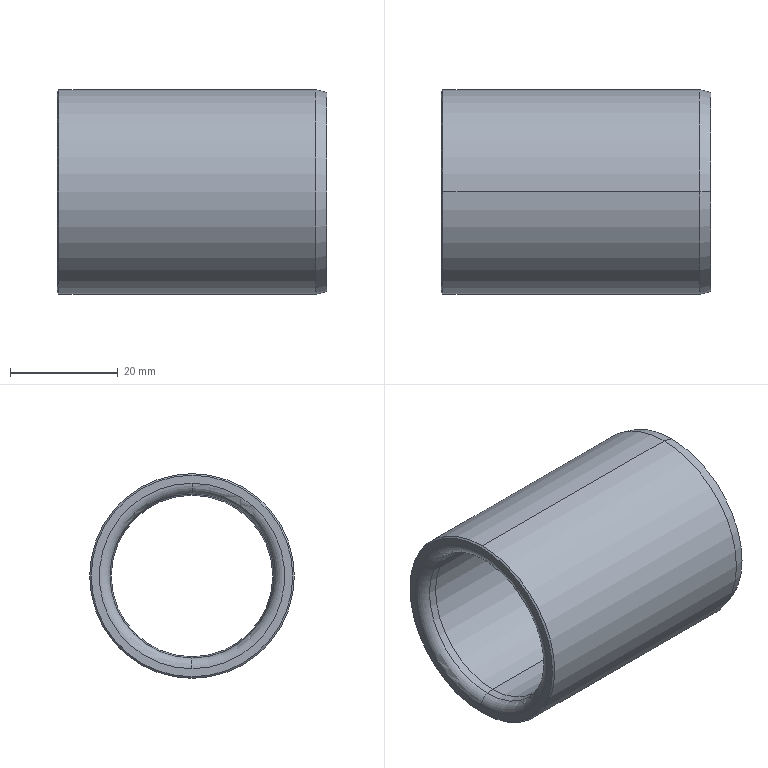Part | STEP file | MPBZ30_50_MPBZ30-50 | 1 solid | 18 faces | box 50 x 38 x 38 mm | volume 21031 mm3 | cone 8 | cylinder 4 | torus 4 | plane 2 | commonest cylinder face diameters 30 x2 38 x2
STEP:
#1=CARTESIAN_POINT('',(0.,0.,0.));
#2=DIRECTION('',(0.,0.,1.));
#3=DIRECTION('',(1.,0.,0.));
#4=AXIS2_PLACEMENT_3D('',#1,#2,#3);
#5=CARTESIAN_POINT('',(48.,0.,19.));
#6=VERTEX_POINT('',#5);
#7=CARTESIAN_POINT('',(48.,0.,-19.));
#8=VERTEX_POINT('',#7);
#9=CARTESIAN_POINT('',(48.,0.,0.));
#10=DIRECTION('',(-1.,0.,0.));
#11=DIRECTION('',(0.,0.,1.));
#12=AXIS2_PLACEMENT_3D('',#9,#10,#11);
#13=CIRCLE('',#12,19.);
#14=CARTESIAN_POINT('',(50.,0.,0.));
#15=DIRECTION('',(-1.,0.,0.));
#16=DIRECTION('',(0.,0.,1.));
#17=AXIS2_PLACEMENT_3D('',#14,#15,#16);
#18=CYLINDRICAL_SURFACE('',#17,19.);
#19=CARTESIAN_POINT('',(0.,2.));
#20=DIRECTION('',(1.,0.));
#21=VECTOR('',#20,1.);
#22=LINE('',#19,#21);
#23=(GEOMETRIC_REPRESENTATION_CONTEXT(2)PARAMETRIC_REPRESENTATION_CONTEXT()REPRESENTATION_CONTEXT('',''));
#24=DEFINITIONAL_REPRESENTATION('',(#22),#23);
#25=PCURVE('',#18,#24);
#26=CARTESIAN_POINT('',(50.,0.,0.));
#27=DIRECTION('',(-1.,0.,0.));
#28=DIRECTION('',(0.,0.,1.));
#29=AXIS2_PLACEMENT_3D('',#26,#27,#28);
#30=CONICAL_SURFACE('',#29,18.464,0.2618);
#31=CARTESIAN_POINT('',(0.,2.));
#32=DIRECTION('',(1.,0.));
#33=VECTOR('',#32,1.);
#34=LINE('',#31,#33);
#35=(GEOMETRIC_REPRESENTATION_CONTEXT(2)PARAMETRIC_REPRESENTATION_CONTEXT()REPRESENTATION_CONTEXT('',''));
#36=DEFINITIONAL_REPRESENTATION('',(#34),#35);
#37=PCURVE('',#30,#36);
#38=SURFACE_CURVE('',#13,(#25,#37),.PCURVE_S1.);
#39=EDGE_CURVE('',#6,#8,#38,.T.);
#40=ORIENTED_EDGE('',*,*,#39,.T.);
#41=CARTESIAN_POINT('',(0.3,0.,-19.));
#42=VERTEX_POINT('',#41);
#43=CARTESIAN_POINT('',(50.,0.,-19.));
#44=DIRECTION('',(-1.,0.,0.));
#45=VECTOR('',#44,1.);
#46=LINE('',#43,#45);
#47=CARTESIAN_POINT('',(3.142,0.));
#48=DIRECTION('',(0.,1.));
#49=VECTOR('',#48,1.);
#50=LINE('',#47,#49);
#51=(GEOMETRIC_REPRESENTATION_CONTEXT(2)PARAMETRIC_REPRESENTATION_CONTEXT()REPRESENTATION_CONTEXT('',''));
#52=DEFINITIONAL_REPRESENTATION('',(#50),#51);
#53=PCURVE('',#18,#52);
#54=CARTESIAN_POINT('',(50.,0.,0.));
#55=DIRECTION('',(-1.,0.,0.));
#56=DIRECTION('',(0.,0.,1.));
#57=AXIS2_PLACEMENT_3D('',#54,#55,#56);
#58=CYLINDRICAL_SURFACE('',#57,19.);
#59=CARTESIAN_POINT('',(3.142,0.));
#60=DIRECTION('',(0.,1.));
#61=VECTOR('',#60,1.);
#62=LINE('',#59,#61);
#63=(GEOMETRIC_REPRESENTATION_CONTEXT(2)PARAMETRIC_REPRESENTATION_CONTEXT()REPRESENTATION_CONTEXT('',''));
#64=DEFINITIONAL_REPRESENTATION('',(#62),#63);
#65=PCURVE('',#58,#64);
#66=SURFACE_CURVE('',#46,(#53,#65),.PCURVE_S1.);
#67=EDGE_CURVE('',#8,#42,#66,.T.);
#68=ORIENTED_EDGE('',*,*,#67,.T.);
#69=CARTESIAN_POINT('',(0.3,0.,19.));
#70=VERTEX_POINT('',#69);
#71=CARTESIAN_POINT('',(0.3,0.,0.));
#72=DIRECTION('',(-1.,0.,0.));
#73=DIRECTION('',(0.,0.,1.));
#74=AXIS2_PLACEMENT_3D('',#71,#72,#73);
#75=CIRCLE('',#74,19.);
#76=CARTESIAN_POINT('',(0.,49.7));
#77=DIRECTION('',(1.,0.));
#78=VECTOR('',#77,1.);
#79=LINE('',#76,#78);
#80=(GEOMETRIC_REPRESENTATION_CONTEXT(2)PARAMETRIC_REPRESENTATION_CONTEXT()REPRESENTATION_CONTEXT('',''));
#81=DEFINITIONAL_REPRESENTATION('',(#79),#80);
#82=PCURVE('',#18,#81);
#83=CARTESIAN_POINT('',(0.3,0.,0.));
#84=DIRECTION('',(1.,0.,0.));
#85=DIRECTION('',(0.,0.,-1.));
#86=AXIS2_PLACEMENT_3D('',#83,#84,#85);
#87=CONICAL_SURFACE('',#86,19.,0.7854);
#88=CARTESIAN_POINT('',(3.142,0.));
#89=DIRECTION('',(-1.,0.));
#90=VECTOR('',#89,1.);
#91=LINE('',#88,#90);
#92=(GEOMETRIC_REPRESENTATION_CONTEXT(2)PARAMETRIC_REPRESENTATION_CONTEXT()REPRESENTATION_CONTEXT('',''));
#93=DEFINITIONAL_REPRESENTATION('',(#91),#92);
#94=PCURVE('',#87,#93);
#95=SURFACE_CURVE('',#75,(#82,#94),.PCURVE_S1.);
#96=EDGE_CURVE('',#70,#42,#95,.T.);
#97=ORIENTED_EDGE('',*,*,#96,.F.);
#98=CARTESIAN_POINT('',(50.,0.,19.));
#99=DIRECTION('',(-1.,0.,0.));
#100=VECTOR('',#99,1.);
#101=LINE('',#98,#100);
#102=CARTESIAN_POINT('',(0.,0.));
#103=DIRECTION('',(0.,1.));
#104=VECTOR('',#103,1.);
#105=LINE('',#102,#104);
#106=(GEOMETRIC_REPRESENTATION_CONTEXT(2)PARAMETRIC_REPRESENTATION_CONTEXT()REPRESENTATION_CONTEXT('',''));
#107=DEFINITIONAL_REPRESENTATION('',(#105),#106);
#108=PCURVE('',#18,#107);
#109=CARTESIAN_POINT('',(6.283,0.));
#110=DIRECTION('',(0.,1.));
#111=VECTOR('',#110,1.);
#112=LINE('',#109,#111);
#113=(GEOMETRIC_REPRESENTATION_CONTEXT(2)PARAMETRIC_REPRESENTATION_CONTEXT()REPRESENTATION_CONTEXT('',''));
#114=DEFINITIONAL_REPRESENTATION('',(#112),#113);
#115=PCURVE('',#58,#114);
#116=SURFACE_CURVE('',#101,(#108,#115),.PCURVE_S1.);
#117=EDGE_CURVE('',#6,#70,#116,.T.);
#118=ORIENTED_EDGE('',*,*,#117,.F.);
#119=EDGE_LOOP('',(#40,#68,#97,#118));
#120=FACE_BOUND('',#119,.T.);
#121=ADVANCED_FACE('',(#120),#18,.T.);
#122=CARTESIAN_POINT('',(50.,0.,18.464));
#123=VERTEX_POINT('',#122);
#124=CARTESIAN_POINT('',(50.,0.,-18.464));
#125=VERTEX_POINT('',#124);
#126=CARTESIAN_POINT('',(50.,0.,0.));
#127=DIRECTION('',(-1.,0.,0.));
#128=DIRECTION('',(0.,0.,1.));
#129=AXIS2_PLACEMENT_3D('',#126,#127,#128);
#130=CIRCLE('',#129,18.464);
#131=CARTESIAN_POINT('',(0.,0.));
#132=DIRECTION('',(1.,0.));
#133=VECTOR('',#132,1.);
#134=LINE('',#131,#133);
#135=(GEOMETRIC_REPRESENTATION_CONTEXT(2)PARAMETRIC_REPRESENTATION_CONTEXT()REPRESENTATION_CONTEXT('',''));
#136=DEFINITIONAL_REPRESENTATION('',(#134),#135);
#137=PCURVE('',#30,#136);
#138=CARTESIAN_POINT('',(50.,17.207,0.));
#139=DIRECTION('',(-1.,0.,0.));
#140=DIRECTION('',(0.,0.,1.));
#141=AXIS2_PLACEMENT_3D('',#138,#139,#140);
#142=PLANE('',#141);
#143=CARTESIAN_POINT('',(0.,-17.207));
#144=DIRECTION('',(1.,0.));
#145=AXIS2_PLACEMENT_2D('',#143,#144);
#146=CIRCLE('',#145,18.464);
#147=(GEOMETRIC_REPRESENTATION_CONTEXT(2)PARAMETRIC_REPRESENTATION_CONTEXT()REPRESENTATION_CONTEXT('',''));
#148=DEFINITIONAL_REPRESENTATION('',(#146),#147);
#149=PCURVE('',#142,#148);
#150=SURFACE_CURVE('',#130,(#137,#149),.PCURVE_S1.);
#151=EDGE_CURVE('',#123,#125,#150,.T.);
#152=ORIENTED_EDGE('',*,*,#151,.T.);
#153=CARTESIAN_POINT('',(50.,0.,-18.464));
#154=DIRECTION('',(-0.9659,0.,-0.2588));
#155=VECTOR('',#154,1.);
#156=LINE('',#153,#155);
#157=CARTESIAN_POINT('',(3.142,0.));
#158=DIRECTION('',(0.,1.));
#159=VECTOR('',#158,1.);
#160=LINE('',#157,#159);
#161=(GEOMETRIC_REPRESENTATION_CONTEXT(2)PARAMETRIC_REPRESENTATION_CONTEXT()REPRESENTATION_CONTEXT('',''));
#162=DEFINITIONAL_REPRESENTATION('',(#160),#161);
#163=PCURVE('',#30,#162);
#164=CARTESIAN_POINT('',(50.,0.,0.));
#165=DIRECTION('',(-1.,0.,0.));
#166=DIRECTION('',(0.,0.,1.));
#167=AXIS2_PLACEMENT_3D('',#164,#165,#166);
#168=CONICAL_SURFACE('',#167,18.464,0.2618);
#169=CARTESIAN_POINT('',(3.142,0.));
#170=DIRECTION('',(0.,1.));
#171=VECTOR('',#170,1.);
#172=LINE('',#169,#171);
#173=(GEOMETRIC_REPRESENTATION_CONTEXT(2)PARAMETRIC_REPRESENTATION_CONTEXT()REPRESENTATION_CONTEXT('',''));
#174=DEFINITIONAL_REPRESENTATION('',(#172),#173);
#175=PCURVE('',#168,#174);
#176=SURFACE_CURVE('',#156,(#163,#175),.PCURVE_S1.);
#177=EDGE_CURVE('',#125,#8,#176,.T.);
#178=ORIENTED_EDGE('',*,*,#177,.T.);
#179=ORIENTED_EDGE('',*,*,#39,.F.);
#180=CARTESIAN_POINT('',(50.,0.,18.464));
#181=DIRECTION('',(-0.9659,0.,0.2588));
#182=VECTOR('',#181,1.);
#183=LINE('',#180,#182);
#184=CARTESIAN_POINT('',(0.,0.));
#185=DIRECTION('',(0.,1.));
#186=VECTOR('',#185,1.);
#187=LINE('',#184,#186);
#188=(GEOMETRIC_REPRESENTATION_CONTEXT(2)PARAMETRIC_REPRESENTATION_CONTEXT()REPRESENTATION_CONTEXT('',''));
#189=DEFINITIONAL_REPRESENTATION('',(#187),#188);
#190=PCURVE('',#30,#189);
#191=CARTESIAN_POINT('',(6.283,0.));
#192=DIRECTION('',(0.,1.));
#193=VECTOR('',#192,1.);
#194=LINE('',#191,#193);
#195=(GEOMETRIC_REPRESENTATION_CONTEXT(2)PARAMETRIC_REPRESENTATION_CONTEXT()REPRESENTATION_CONTEXT('',''));
#196=DEFINITIONAL_REPRESENTATION('',(#194),#195);
#197=PCURVE('',#168,#196);
#198=SURFACE_CURVE('',#183,(#190,#197),.PCURVE_S1.);
#199=EDGE_CURVE('',#123,#6,#198,.T.);
#200=ORIENTED_EDGE('',*,*,#199,.F.);
#201=EDGE_LOOP('',(#152,#178,#179,#200));
#202=FACE_BOUND('',#201,.T.);
#203=ADVANCED_FACE('',(#202),#30,.T.);
#204=CARTESIAN_POINT('',(48.347,0.,15.238));
#205=VERTEX_POINT('',#204);
#206=CARTESIAN_POINT('',(48.347,0.,-15.238));
#207=VERTEX_POINT('',#206);
#208=CARTESIAN_POINT('',(48.347,0.,0.));
#209=DIRECTION('',(-1.,0.,0.));
#210=DIRECTION('',(0.,0.,1.));
#211=AXIS2_PLACEMENT_3D('',#208,#209,#210);
#212=CIRCLE('',#211,15.238);
#213=CARTESIAN_POINT('',(48.,0.,0.));
#214=DIRECTION('',(-1.,0.,0.));
#215=DIRECTION('',(0.,0.,1.));
#216=AXIS2_PLACEMENT_3D('',#213,#214,#215);
#217=TOROIDAL_SURFACE('',#216,17.207,2.);
#218=CARTESIAN_POINT('',(0.,3.316));
#219=DIRECTION('',(1.,0.));
#220=VECTOR('',#219,1.);
#221=LINE('',#218,#220);
#222=(GEOMETRIC_REPRESENTATION_CONTEXT(2)PARAMETRIC_REPRESENTATION_CONTEXT()REPRESENTATION_CONTEXT('',''));
#223=DEFINITIONAL_REPRESENTATION('',(#221),#222);
#224=PCURVE('',#217,#223);
#225=CARTESIAN_POINT('',(47.,0.,0.));
#226=DIRECTION('',(1.,0.,0.));
#227=DIRECTION('',(0.,0.,-1.));
#228=AXIS2_PLACEMENT_3D('',#225,#226,#227);
#229=CONICAL_SURFACE('',#228,15.,0.1745);
#230=CARTESIAN_POINT('',(3.142,1.347));
#231=DIRECTION('',(-1.,0.));
#232=VECTOR('',#231,1.);
#233=LINE('',#230,#232);
#234=(GEOMETRIC_REPRESENTATION_CONTEXT(2)PARAMETRIC_REPRESENTATION_CONTEXT()REPRESENTATION_CONTEXT('',''));
#235=DEFINITIONAL_REPRESENTATION('',(#233),#234);
#236=PCURVE('',#229,#235);
#237=SURFACE_CURVE('',#212,(#224,#236),.PCURVE_S1.);
#238=EDGE_CURVE('',#205,#207,#237,.T.);
#239=ORIENTED_EDGE('',*,*,#238,.T.);
#240=CARTESIAN_POINT('',(50.,0.,-17.207));
#241=VERTEX_POINT('',#240);
#242=CARTESIAN_POINT('',(48.,0.,-17.207));
#243=DIRECTION('',(0.,1.,0.));
#244=DIRECTION('',(0.,0.,1.));
#245=AXIS2_PLACEMENT_3D('',#242,#243,#244);
#246=CIRCLE('',#245,2.);
#247=CARTESIAN_POINT('',(3.142,3.142));
#248=DIRECTION('',(0.,1.));
#249=VECTOR('',#248,1.);
#250=LINE('',#247,#249);
#251=(GEOMETRIC_REPRESENTATION_CONTEXT(2)PARAMETRIC_REPRESENTATION_CONTEXT()REPRESENTATION_CONTEXT('',''));
#252=DEFINITIONAL_REPRESENTATION('',(#250),#251);
#253=PCURVE('',#217,#252);
#254=CARTESIAN_POINT('',(48.,0.,0.));
#255=DIRECTION('',(-1.,0.,0.));
#256=DIRECTION('',(0.,0.,1.));
#257=AXIS2_PLACEMENT_3D('',#254,#255,#256);
#258=TOROIDAL_SURFACE('',#257,17.207,2.);
#259=CARTESIAN_POINT('',(3.142,3.142));
#260=DIRECTION('',(0.,1.));
#261=VECTOR('',#260,1.);
#262=LINE('',#259,#261);
#263=(GEOMETRIC_REPRESENTATION_CONTEXT(2)PARAMETRIC_REPRESENTATION_CONTEXT()REPRESENTATION_CONTEXT('',''));
#264=DEFINITIONAL_REPRESENTATION('',(#262),#263);
#265=PCURVE('',#258,#264);
#266=SURFACE_CURVE('',#246,(#253,#265),.PCURVE_S1.);
#267=EDGE_CURVE('',#207,#241,#266,.T.);
#268=ORIENTED_EDGE('',*,*,#267,.T.);
#269=CARTESIAN_POINT('',(50.,0.,17.207));
#270=VERTEX_POINT('',#269);
#271=CARTESIAN_POINT('',(50.,0.,0.));
#272=DIRECTION('',(-1.,0.,0.));
#273=DIRECTION('',(0.,0.,1.));
#274=AXIS2_PLACEMENT_3D('',#271,#272,#273);
#275=CIRCLE('',#274,17.207);
#276=CARTESIAN_POINT('',(0.,4.712));
#277=DIRECTION('',(1.,0.));
#278=VECTOR('',#277,1.);
#279=LINE('',#276,#278);
#280=(GEOMETRIC_REPRESENTATION_CONTEXT(2)PARAMETRIC_REPRESENTATION_CONTEXT()REPRESENTATION_CONTEXT('',''));
#281=DEFINITIONAL_REPRESENTATION('',(#279),#280);
#282=PCURVE('',#217,#281);
#283=CARTESIAN_POINT('',(0.,-17.207));
#284=DIRECTION('',(1.,0.));
#285=AXIS2_PLACEMENT_2D('',#283,#284);
#286=CIRCLE('',#285,17.207);
#287=(GEOMETRIC_REPRESENTATION_CONTEXT(2)PARAMETRIC_REPRESENTATION_CONTEXT()REPRESENTATION_CONTEXT('',''));
#288=DEFINITIONAL_REPRESENTATION('',(#286),#287);
#289=PCURVE('',#142,#288);
#290=SURFACE_CURVE('',#275,(#282,#289),.PCURVE_S1.);
#291=EDGE_CURVE('',#270,#241,#290,.T.);
#292=ORIENTED_EDGE('',*,*,#291,.F.);
#293=CARTESIAN_POINT('',(48.,0.,17.207));
#294=DIRECTION('',(0.,-1.,0.));
#295=DIRECTION('',(0.,0.,-1.));
#296=AXIS2_PLACEMENT_3D('',#293,#294,#295);
#297=CIRCLE('',#296,2.);
#298=CARTESIAN_POINT('',(0.,3.142));
#299=DIRECTION('',(0.,1.));
#300=VECTOR('',#299,1.);
#301=LINE('',#298,#300);
#302=(GEOMETRIC_REPRESENTATION_CONTEXT(2)PARAMETRIC_REPRESENTATION_CONTEXT()REPRESENTATION_CONTEXT('',''));
#303=DEFINITIONAL_REPRESENTATION('',(#301),#302);
#304=PCURVE('',#217,#303);
#305=CARTESIAN_POINT('',(6.283,3.142));
#306=DIRECTION('',(0.,1.));
#307=VECTOR('',#306,1.);
#308=LINE('',#305,#307);
#309=(GEOMETRIC_REPRESENTATION_CONTEXT(2)PARAMETRIC_REPRESENTATION_CONTEXT()REPRESENTATION_CONTEXT('',''));
#310=DEFINITIONAL_REPRESENTATION('',(#308),#309);
#311=PCURVE('',#258,#310);
#312=SURFACE_CURVE('',#297,(#304,#311),.PCURVE_S1.);
#313=EDGE_CURVE('',#205,#270,#312,.T.);
#314=ORIENTED_EDGE('',*,*,#313,.F.);
#315=EDGE_LOOP('',(#239,#268,#292,#314));
#316=FACE_BOUND('',#315,.T.);
#317=ADVANCED_FACE('',(#316),#217,.T.);
#318=CARTESIAN_POINT('',(47.,0.,-15.));
#319=VERTEX_POINT('',#318);
#320=CARTESIAN_POINT('',(47.,0.,-15.));
#321=DIRECTION('',(0.9848,0.,-0.1736));
#322=VECTOR('',#321,1.);
#323=LINE('',#320,#322);
#324=CARTESIAN_POINT('',(47.,0.,0.));
#325=DIRECTION('',(1.,0.,0.));
#326=DIRECTION('',(0.,0.,-1.));
#327=AXIS2_PLACEMENT_3D('',#324,#325,#326);
#328=CONICAL_SURFACE('',#327,15.,0.1745);
#329=CARTESIAN_POINT('',(6.283,0.));
#330=DIRECTION('',(0.,1.));
#331=VECTOR('',#330,1.);
#332=LINE('',#329,#331);
#333=(GEOMETRIC_REPRESENTATION_CONTEXT(2)PARAMETRIC_REPRESENTATION_CONTEXT()REPRESENTATION_CONTEXT('',''));
#334=DEFINITIONAL_REPRESENTATION('',(#332),#333);
#335=PCURVE('',#328,#334);
#336=CARTESIAN_POINT('',(0.,0.));
#337=DIRECTION('',(0.,1.));
#338=VECTOR('',#337,1.);
#339=LINE('',#336,#338);
#340=(GEOMETRIC_REPRESENTATION_CONTEXT(2)PARAMETRIC_REPRESENTATION_CONTEXT()REPRESENTATION_CONTEXT('',''));
#341=DEFINITIONAL_REPRESENTATION('',(#339),#340);
#342=PCURVE('',#229,#341);
#343=SURFACE_CURVE('',#323,(#335,#342),.PCURVE_S1.);
#344=EDGE_CURVE('',#319,#207,#343,.T.);
#345=ORIENTED_EDGE('',*,*,#344,.T.);
#346=CARTESIAN_POINT('',(48.347,0.,0.));
#347=DIRECTION('',(-1.,0.,0.));
#348=DIRECTION('',(0.,0.,1.));
#349=AXIS2_PLACEMENT_3D('',#346,#347,#348);
#350=CIRCLE('',#349,15.238);
#351=CARTESIAN_POINT('',(9.425,1.347));
#352=DIRECTION('',(-1.,0.));
#353=VECTOR('',#352,1.);
#354=LINE('',#351,#353);
#355=(GEOMETRIC_REPRESENTATION_CONTEXT(2)PARAMETRIC_REPRESENTATION_CONTEXT()REPRESENTATION_CONTEXT('',''));
#356=DEFINITIONAL_REPRESENTATION('',(#354),#355);
#357=PCURVE('',#328,#356);
#358=CARTESIAN_POINT('',(0.,3.316));
#359=DIRECTION('',(1.,0.));
#360=VECTOR('',#359,1.);
#361=LINE('',#358,#360);
#362=(GEOMETRIC_REPRESENTATION_CONTEXT(2)PARAMETRIC_REPRESENTATION_CONTEXT()REPRESENTATION_CONTEXT('',''));
#363=DEFINITIONAL_REPRESENTATION('',(#361),#362);
#364=PCURVE('',#258,#363);
#365=SURFACE_CURVE('',#350,(#357,#364),.PCURVE_S1.);
#366=EDGE_CURVE('',#207,#205,#365,.T.);
#367=ORIENTED_EDGE('',*,*,#366,.T.);
#368=CARTESIAN_POINT('',(47.,0.,15.));
#369=VERTEX_POINT('',#368);
#370=CARTESIAN_POINT('',(47.,0.,15.));
#371=DIRECTION('',(0.9848,0.,0.1736));
#372=VECTOR('',#371,1.);
#373=LINE('',#370,#372);
#374=CARTESIAN_POINT('',(3.142,0.));
#375=DIRECTION('',(0.,1.));
#376=VECTOR('',#375,1.);
#377=LINE('',#374,#376);
#378=(GEOMETRIC_REPRESENTATION_CONTEXT(2)PARAMETRIC_REPRESENTATION_CONTEXT()REPRESENTATION_CONTEXT('',''));
#379=DEFINITIONAL_REPRESENTATION('',(#377),#378);
#380=PCURVE('',#328,#379);
#381=CARTESIAN_POINT('',(3.142,0.));
#382=DIRECTION('',(0.,1.));
#383=VECTOR('',#382,1.);
#384=LINE('',#381,#383);
#385=(GEOMETRIC_REPRESENTATION_CONTEXT(2)PARAMETRIC_REPRESENTATION_CONTEXT()REPRESENTATION_CONTEXT('',''));
#386=DEFINITIONAL_REPRESENTATION('',(#384),#385);
#387=PCURVE('',#229,#386);
#388=SURFACE_CURVE('',#373,(#380,#387),.PCURVE_S1.);
#389=EDGE_CURVE('',#369,#205,#388,.T.);
#390=ORIENTED_EDGE('',*,*,#389,.F.);
#391=CARTESIAN_POINT('',(47.,0.,0.));
#392=DIRECTION('',(-1.,0.,0.));
#393=DIRECTION('',(0.,0.,1.));
#394=AXIS2_PLACEMENT_3D('',#391,#392,#393);
#395=CIRCLE('',#394,15.);
#396=CARTESIAN_POINT('',(9.425,0.));
#397=DIRECTION('',(-1.,0.));
#398=VECTOR('',#397,1.);
#399=LINE('',#396,#398);
#400=(GEOMETRIC_REPRESENTATION_CONTEXT(2)PARAMETRIC_REPRESENTATION_CONTEXT()REPRESENTATION_CONTEXT('',''));
#401=DEFINITIONAL_REPRESENTATION('',(#399),#400);
#402=PCURVE('',#328,#401);
#403=CARTESIAN_POINT('',(50.,0.,0.));
#404=DIRECTION('',(-1.,0.,0.));
#405=DIRECTION('',(0.,0.,1.));
#406=AXIS2_PLACEMENT_3D('',#403,#404,#405);
#407=CYLINDRICAL_SURFACE('',#406,15.);
#408=CARTESIAN_POINT('',(0.,3.));
#409=DIRECTION('',(1.,0.));
#410=VECTOR('',#409,1.);
#411=LINE('',#408,#410);
#412=(GEOMETRIC_REPRESENTATION_CONTEXT(2)PARAMETRIC_REPRESENTATION_CONTEXT()REPRESENTATION_CONTEXT('',''));
#413=DEFINITIONAL_REPRESENTATION('',(#411),#412);
#414=PCURVE('',#407,#413);
#415=SURFACE_CURVE('',#395,(#402,#414),.PCURVE_S1.);
#416=EDGE_CURVE('',#319,#369,#415,.T.);
#417=ORIENTED_EDGE('',*,*,#416,.F.);
#418=EDGE_LOOP('',(#345,#367,#390,#417));
#419=FACE_BOUND('',#418,.F.);
#420=ADVANCED_FACE('',(#419),#328,.F.);
#421=CARTESIAN_POINT('',(3.,0.,15.));
#422=VERTEX_POINT('',#421);
#423=CARTESIAN_POINT('',(50.,0.,15.));
#424=DIRECTION('',(-1.,0.,0.));
#425=VECTOR('',#424,1.);
#426=LINE('',#423,#425);
#427=CARTESIAN_POINT('',(6.283,0.));
#428=DIRECTION('',(0.,1.));
#429=VECTOR('',#428,1.);
#430=LINE('',#427,#429);
#431=(GEOMETRIC_REPRESENTATION_CONTEXT(2)PARAMETRIC_REPRESENTATION_CONTEXT()REPRESENTATION_CONTEXT('',''));
#432=DEFINITIONAL_REPRESENTATION('',(#430),#431);
#433=PCURVE('',#407,#432);
#434=CARTESIAN_POINT('',(50.,0.,0.));
#435=DIRECTION('',(-1.,0.,0.));
#436=DIRECTION('',(0.,0.,1.));
#437=AXIS2_PLACEMENT_3D('',#434,#435,#436);
#438=CYLINDRICAL_SURFACE('',#437,15.);
#439=CARTESIAN_POINT('',(0.,0.));
#440=DIRECTION('',(0.,1.));
#441=VECTOR('',#440,1.);
#442=LINE('',#439,#441);
#443=(GEOMETRIC_REPRESENTATION_CONTEXT(2)PARAMETRIC_REPRESENTATION_CONTEXT()REPRESENTATION_CONTEXT('',''));
#444=DEFINITIONAL_REPRESENTATION('',(#442),#443);
#445=PCURVE('',#438,#444);
#446=SURFACE_CURVE('',#426,(#433,#445),.PCURVE_S1.);
#447=EDGE_CURVE('',#369,#422,#446,.T.);
#448=ORIENTED_EDGE('',*,*,#447,.T.);
#449=CARTESIAN_POINT('',(3.,0.,-15.));
#450=VERTEX_POINT('',#449);
#451=CARTESIAN_POINT('',(3.,0.,0.));
#452=DIRECTION('',(-1.,0.,0.));
#453=DIRECTION('',(0.,0.,1.));
#454=AXIS2_PLACEMENT_3D('',#451,#452,#453);
#455=CIRCLE('',#454,15.);
#456=CARTESIAN_POINT('',(0.,47.));
#457=DIRECTION('',(1.,0.));
#458=VECTOR('',#457,1.);
#459=LINE('',#456,#458);
#460=(GEOMETRIC_REPRESENTATION_CONTEXT(2)PARAMETRIC_REPRESENTATION_CONTEXT()REPRESENTATION_CONTEXT('',''));
#461=DEFINITIONAL_REPRESENTATION('',(#459),#460);
#462=PCURVE('',#407,#461);
#463=CARTESIAN_POINT('',(1.653,0.,0.));
#464=DIRECTION('',(-1.,0.,0.));
#465=DIRECTION('',(0.,0.,1.));
#466=AXIS2_PLACEMENT_3D('',#463,#464,#465);
#467=CONICAL_SURFACE('',#466,15.238,0.1745);
#468=CARTESIAN_POINT('',(0.,-1.347));
#469=DIRECTION('',(1.,0.));
#470=VECTOR('',#469,1.);
#471=LINE('',#468,#470);
#472=(GEOMETRIC_REPRESENTATION_CONTEXT(2)PARAMETRIC_REPRESENTATION_CONTEXT()REPRESENTATION_CONTEXT('',''));
#473=DEFINITIONAL_REPRESENTATION('',(#471),#472);
#474=PCURVE('',#467,#473);
#475=SURFACE_CURVE('',#455,(#462,#474),.PCURVE_S1.);
#476=EDGE_CURVE('',#450,#422,#475,.T.);
#477=ORIENTED_EDGE('',*,*,#476,.F.);
#478=CARTESIAN_POINT('',(50.,0.,-15.));
#479=DIRECTION('',(-1.,0.,0.));
#480=VECTOR('',#479,1.);
#481=LINE('',#478,#480);
#482=CARTESIAN_POINT('',(3.142,0.));
#483=DIRECTION('',(0.,1.));
#484=VECTOR('',#483,1.);
#485=LINE('',#482,#484);
#486=(GEOMETRIC_REPRESENTATION_CONTEXT(2)PARAMETRIC_REPRESENTATION_CONTEXT()REPRESENTATION_CONTEXT('',''));
#487=DEFINITIONAL_REPRESENTATION('',(#485),#486);
#488=PCURVE('',#407,#487);
#489=CARTESIAN_POINT('',(3.142,0.));
#490=DIRECTION('',(0.,1.));
#491=VECTOR('',#490,1.);
#492=LINE('',#489,#491);
#493=(GEOMETRIC_REPRESENTATION_CONTEXT(2)PARAMETRIC_REPRESENTATION_CONTEXT()REPRESENTATION_CONTEXT('',''));
#494=DEFINITIONAL_REPRESENTATION('',(#492),#493);
#495=PCURVE('',#438,#494);
#496=SURFACE_CURVE('',#481,(#488,#495),.PCURVE_S1.);
#497=EDGE_CURVE('',#319,#450,#496,.T.);
#498=ORIENTED_EDGE('',*,*,#497,.F.);
#499=ORIENTED_EDGE('',*,*,#416,.T.);
#500=EDGE_LOOP('',(#448,#477,#498,#499));
#501=FACE_BOUND('',#500,.F.);
#502=ADVANCED_FACE('',(#501),#407,.F.);
#503=CARTESIAN_POINT('',(1.653,0.,15.238));
#504=VERTEX_POINT('',#503);
#505=CARTESIAN_POINT('',(1.653,0.,15.238));
#506=DIRECTION('',(-0.9848,0.,0.1736));
#507=VECTOR('',#506,1.);
#508=LINE('',#505,#507);
#509=CARTESIAN_POINT('',(6.283,0.));
#510=DIRECTION('',(0.,1.));
#511=VECTOR('',#510,1.);
#512=LINE('',#509,#511);
#513=(GEOMETRIC_REPRESENTATION_CONTEXT(2)PARAMETRIC_REPRESENTATION_CONTEXT()REPRESENTATION_CONTEXT('',''));
#514=DEFINITIONAL_REPRESENTATION('',(#512),#513);
#515=PCURVE('',#467,#514);
#516=CARTESIAN_POINT('',(1.653,0.,0.));
#517=DIRECTION('',(-1.,0.,0.));
#518=DIRECTION('',(0.,0.,1.));
#519=AXIS2_PLACEMENT_3D('',#516,#517,#518);
#520=CONICAL_SURFACE('',#519,15.238,0.1745);
#521=CARTESIAN_POINT('',(0.,0.));
#522=DIRECTION('',(0.,1.));
#523=VECTOR('',#522,1.);
#524=LINE('',#521,#523);
#525=(GEOMETRIC_REPRESENTATION_CONTEXT(2)PARAMETRIC_REPRESENTATION_CONTEXT()REPRESENTATION_CONTEXT('',''));
#526=DEFINITIONAL_REPRESENTATION('',(#524),#525);
#527=PCURVE('',#520,#526);
#528=SURFACE_CURVE('',#508,(#515,#527),.PCURVE_S1.);
#529=EDGE_CURVE('',#422,#504,#528,.T.);
#530=ORIENTED_EDGE('',*,*,#529,.T.);
#531=CARTESIAN_POINT('',(1.653,0.,-15.238));
#532=VERTEX_POINT('',#531);
#533=CARTESIAN_POINT('',(1.653,0.,0.));
#534=DIRECTION('',(-1.,0.,0.));
#535=DIRECTION('',(0.,0.,1.));
#536=AXIS2_PLACEMENT_3D('',#533,#534,#535);
#537=CIRCLE('',#536,15.238);
#538=CARTESIAN_POINT('',(0.,0.));
#539=DIRECTION('',(1.,0.));
#540=VECTOR('',#539,1.);
#541=LINE('',#538,#540);
#542=(GEOMETRIC_REPRESENTATION_CONTEXT(2)PARAMETRIC_REPRESENTATION_CONTEXT()REPRESENTATION_CONTEXT('',''));
#543=DEFINITIONAL_REPRESENTATION('',(#541),#542);
#544=PCURVE('',#467,#543);
#545=CARTESIAN_POINT('',(2.,0.,0.));
#546=DIRECTION('',(-1.,0.,0.));
#547=DIRECTION('',(0.,0.,1.));
#548=AXIS2_PLACEMENT_3D('',#545,#546,#547);
#549=TOROIDAL_SURFACE('',#548,17.207,2.);
#550=CARTESIAN_POINT('',(0.,2.967));
#551=DIRECTION('',(1.,0.));
#552=VECTOR('',#551,1.);
#553=LINE('',#550,#552);
#554=(GEOMETRIC_REPRESENTATION_CONTEXT(2)PARAMETRIC_REPRESENTATION_CONTEXT()REPRESENTATION_CONTEXT('',''));
#555=DEFINITIONAL_REPRESENTATION('',(#553),#554);
#556=PCURVE('',#549,#555);
#557=SURFACE_CURVE('',#537,(#544,#556),.PCURVE_S1.);
#558=EDGE_CURVE('',#532,#504,#557,.T.);
#559=ORIENTED_EDGE('',*,*,#558,.F.);
#560=CARTESIAN_POINT('',(1.653,0.,-15.238));
#561=DIRECTION('',(-0.9848,0.,-0.1736));
#562=VECTOR('',#561,1.);
#563=LINE('',#560,#562);
#564=CARTESIAN_POINT('',(3.142,0.));
#565=DIRECTION('',(0.,1.));
#566=VECTOR('',#565,1.);
#567=LINE('',#564,#566);
#568=(GEOMETRIC_REPRESENTATION_CONTEXT(2)PARAMETRIC_REPRESENTATION_CONTEXT()REPRESENTATION_CONTEXT('',''));
#569=DEFINITIONAL_REPRESENTATION('',(#567),#568);
#570=PCURVE('',#467,#569);
#571=CARTESIAN_POINT('',(3.142,0.));
#572=DIRECTION('',(0.,1.));
#573=VECTOR('',#572,1.);
#574=LINE('',#571,#573);
#575=(GEOMETRIC_REPRESENTATION_CONTEXT(2)PARAMETRIC_REPRESENTATION_CONTEXT()REPRESENTATION_CONTEXT('',''));
#576=DEFINITIONAL_REPRESENTATION('',(#574),#575);
#577=PCURVE('',#520,#576);
#578=SURFACE_CURVE('',#563,(#570,#577),.PCURVE_S1.);
#579=EDGE_CURVE('',#450,#532,#578,.T.);
#580=ORIENTED_EDGE('',*,*,#579,.F.);
#581=ORIENTED_EDGE('',*,*,#476,.T.);
#582=EDGE_LOOP('',(#530,#559,#580,#581));
#583=FACE_BOUND('',#582,.F.);
#584=ADVANCED_FACE('',(#583),#467,.F.);
#585=CARTESIAN_POINT('',(0.,0.,17.207));
#586=VERTEX_POINT('',#585);
#587=CARTESIAN_POINT('',(0.,0.,-17.207));
#588=VERTEX_POINT('',#587);
#589=CARTESIAN_POINT('',(0.,0.,0.));
#590=DIRECTION('',(-1.,0.,0.));
#591=DIRECTION('',(0.,0.,1.));
#592=AXIS2_PLACEMENT_3D('',#589,#590,#591);
#593=CIRCLE('',#592,17.207);
#594=CARTESIAN_POINT('',(2.,0.,0.));
#595=DIRECTION('',(-1.,0.,0.));
#596=DIRECTION('',(0.,0.,1.));
#597=AXIS2_PLACEMENT_3D('',#594,#595,#596);
#598=TOROIDAL_SURFACE('',#597,17.207,2.);
#599=CARTESIAN_POINT('',(0.,1.571));
#600=DIRECTION('',(1.,0.));
#601=VECTOR('',#600,1.);
#602=LINE('',#599,#601);
#603=(GEOMETRIC_REPRESENTATION_CONTEXT(2)PARAMETRIC_REPRESENTATION_CONTEXT()REPRESENTATION_CONTEXT('',''));
#604=DEFINITIONAL_REPRESENTATION('',(#602),#603);
#605=PCURVE('',#598,#604);
#606=CARTESIAN_POINT('',(0.,18.7,0.));
#607=DIRECTION('',(1.,0.,0.));
#608=DIRECTION('',(0.,0.,-1.));
#609=AXIS2_PLACEMENT_3D('',#606,#607,#608);
#610=PLANE('',#609);
#611=CARTESIAN_POINT('',(-17.207,-18.7));
#612=CARTESIAN_POINT('',(-17.207,11.104));
#613=CARTESIAN_POINT('',(8.604,-3.798));
#614=CARTESIAN_POINT('',(34.414,-18.7));
#615=CARTESIAN_POINT('',(8.604,-33.602));
#616=CARTESIAN_POINT('',(-17.207,-48.504));
#617=CARTESIAN_POINT('',(-17.207,-18.7));
#618=(BOUNDED_CURVE()B_SPLINE_CURVE(2,(#611,#612,#613,#614,#615,#616,#617),.UNSPECIFIED.,.T.,.F.)B_SPLINE_CURVE_WITH_KNOTS((1,2,2,2,2,1),(-2.094,0.,2.094,4.189,6.283,8.378),.UNSPECIFIED.)CURVE()GEOMETRIC_REPRESENTATION_ITEM()RATIONAL_B_SPLINE_CURVE((1.,0.5,1.,0.5,1.,0.5,1.))REPRESENTATION_ITEM(''));
#619=(GEOMETRIC_REPRESENTATION_CONTEXT(2)PARAMETRIC_REPRESENTATION_CONTEXT()REPRESENTATION_CONTEXT('',''));
#620=DEFINITIONAL_REPRESENTATION('',(#618),#619);
#621=PCURVE('',#610,#620);
#622=SURFACE_CURVE('',#593,(#605,#621),.PCURVE_S1.);
#623=EDGE_CURVE('',#586,#588,#622,.T.);
#624=ORIENTED_EDGE('',*,*,#623,.T.);
#625=CARTESIAN_POINT('',(2.,0.,-17.207));
#626=DIRECTION('',(0.,1.,0.));
#627=DIRECTION('',(0.,0.,1.));
#628=AXIS2_PLACEMENT_3D('',#625,#626,#627);
#629=CIRCLE('',#628,2.);
#630=CARTESIAN_POINT('',(3.142,-3.142));
#631=DIRECTION('',(0.,1.));
#632=VECTOR('',#631,1.);
#633=LINE('',#630,#632);
#634=(GEOMETRIC_REPRESENTATION_CONTEXT(2)PARAMETRIC_REPRESENTATION_CONTEXT()REPRESENTATION_CONTEXT('',''));
#635=DEFINITIONAL_REPRESENTATION('',(#633),#634);
#636=PCURVE('',#598,#635);
#637=CARTESIAN_POINT('',(3.142,-3.142));
#638=DIRECTION('',(0.,1.));
#639=VECTOR('',#638,1.);
#640=LINE('',#637,#639);
#641=(GEOMETRIC_REPRESENTATION_CONTEXT(2)PARAMETRIC_REPRESENTATION_CONTEXT()REPRESENTATION_CONTEXT('',''));
#642=DEFINITIONAL_REPRESENTATION('',(#640),#641);
#643=PCURVE('',#549,#642);
#644=SURFACE_CURVE('',#629,(#636,#643),.PCURVE_S1.);
#645=EDGE_CURVE('',#588,#532,#644,.T.);
#646=ORIENTED_EDGE('',*,*,#645,.T.);
#647=CARTESIAN_POINT('',(1.653,0.,0.));
#648=DIRECTION('',(-1.,0.,0.));
#649=DIRECTION('',(0.,0.,1.));
#650=AXIS2_PLACEMENT_3D('',#647,#648,#649);
#651=CIRCLE('',#650,15.238);
#652=CARTESIAN_POINT('',(0.,2.967));
#653=DIRECTION('',(1.,0.));
#654=VECTOR('',#653,1.);
#655=LINE('',#652,#654);
#656=(GEOMETRIC_REPRESENTATION_CONTEXT(2)PARAMETRIC_REPRESENTATION_CONTEXT()REPRESENTATION_CONTEXT('',''));
#657=DEFINITIONAL_REPRESENTATION('',(#655),#656);
#658=PCURVE('',#598,#657);
#659=CARTESIAN_POINT('',(0.,0.));
#660=DIRECTION('',(1.,0.));
#661=VECTOR('',#660,1.);
#662=LINE('',#659,#661);
#663=(GEOMETRIC_REPRESENTATION_CONTEXT(2)PARAMETRIC_REPRESENTATION_CONTEXT()REPRESENTATION_CONTEXT('',''));
#664=DEFINITIONAL_REPRESENTATION('',(#662),#663);
#665=PCURVE('',#520,#664);
#666=SURFACE_CURVE('',#651,(#658,#665),.PCURVE_S1.);
#667=EDGE_CURVE('',#504,#532,#666,.T.);
#668=ORIENTED_EDGE('',*,*,#667,.F.);
#669=CARTESIAN_POINT('',(2.,0.,17.207));
#670=DIRECTION('',(0.,-1.,0.));
#671=DIRECTION('',(0.,0.,-1.));
#672=AXIS2_PLACEMENT_3D('',#669,#670,#671);
#673=CIRCLE('',#672,2.);
#674=CARTESIAN_POINT('',(0.,-3.142));
#675=DIRECTION('',(0.,1.));
#676=VECTOR('',#675,1.);
#677=LINE('',#674,#676);
#678=(GEOMETRIC_REPRESENTATION_CONTEXT(2)PARAMETRIC_REPRESENTATION_CONTEXT()REPRESENTATION_CONTEXT('',''));
#679=DEFINITIONAL_REPRESENTATION('',(#677),#678);
#680=PCURVE('',#598,#679);
#681=CARTESIAN_POINT('',(6.283,-3.142));
#682=DIRECTION('',(0.,1.));
#683=VECTOR('',#682,1.);
#684=LINE('',#681,#683);
#685=(GEOMETRIC_REPRESENTATION_CONTEXT(2)PARAMETRIC_REPRESENTATION_CONTEXT()REPRESENTATION_CONTEXT('',''));
#686=DEFINITIONAL_REPRESENTATION('',(#684),#685);
#687=PCURVE('',#549,#686);
#688=SURFACE_CURVE('',#673,(#680,#687),.PCURVE_S1.);
#689=EDGE_CURVE('',#586,#504,#688,.T.);
#690=ORIENTED_EDGE('',*,*,#689,.F.);
#691=EDGE_LOOP('',(#624,#646,#668,#690));
#692=FACE_BOUND('',#691,.T.);
#693=ADVANCED_FACE('',(#692),#598,.T.);
#694=CARTESIAN_POINT('',(0.,0.,18.7));
#695=VERTEX_POINT('',#694);
#696=CARTESIAN_POINT('',(0.,0.,-18.7));
#697=VERTEX_POINT('',#696);
#698=CARTESIAN_POINT('',(0.,0.,0.));
#699=DIRECTION('',(-1.,0.,0.));
#700=DIRECTION('',(0.,0.,1.));
#701=AXIS2_PLACEMENT_3D('',#698,#699,#700);
#702=CIRCLE('',#701,18.7);
#703=CARTESIAN_POINT('',(3.142,-0.3));
#704=DIRECTION('',(-1.,0.));
#705=VECTOR('',#704,1.);
#706=LINE('',#703,#705);
#707=(GEOMETRIC_REPRESENTATION_CONTEXT(2)PARAMETRIC_REPRESENTATION_CONTEXT()REPRESENTATION_CONTEXT('',''));
#708=DEFINITIONAL_REPRESENTATION('',(#706),#707);
#709=PCURVE('',#87,#708);
#710=CARTESIAN_POINT('',(-18.7,-18.7));
#711=CARTESIAN_POINT('',(-18.7,13.689));
#712=CARTESIAN_POINT('',(9.35,-2.505));
#713=CARTESIAN_POINT('',(37.4,-18.7));
#714=CARTESIAN_POINT('',(9.35,-34.895));
#715=CARTESIAN_POINT('',(-18.7,-51.089));
#716=CARTESIAN_POINT('',(-18.7,-18.7));
#717=(BOUNDED_CURVE()B_SPLINE_CURVE(2,(#710,#711,#712,#713,#714,#715,#716),.UNSPECIFIED.,.T.,.F.)B_SPLINE_CURVE_WITH_KNOTS((1,2,2,2,2,1),(-2.094,0.,2.094,4.189,6.283,8.378),.UNSPECIFIED.)CURVE()GEOMETRIC_REPRESENTATION_ITEM()RATIONAL_B_SPLINE_CURVE((1.,0.5,1.,0.5,1.,0.5,1.))REPRESENTATION_ITEM(''));
#718=(GEOMETRIC_REPRESENTATION_CONTEXT(2)PARAMETRIC_REPRESENTATION_CONTEXT()REPRESENTATION_CONTEXT('',''));
#719=DEFINITIONAL_REPRESENTATION('',(#717),#718);
#720=PCURVE('',#610,#719);
#721=SURFACE_CURVE('',#702,(#709,#720),.PCURVE_S1.);
#722=EDGE_CURVE('',#695,#697,#721,.T.);
#723=ORIENTED_EDGE('',*,*,#722,.F.);
#724=CARTESIAN_POINT('',(0.3,0.,19.));
#725=DIRECTION('',(0.7071,0.,0.7071));
#726=VECTOR('',#725,1.);
#727=LINE('',#724,#726);
#728=CARTESIAN_POINT('',(3.142,0.));
#729=DIRECTION('',(0.,1.));
#730=VECTOR('',#729,1.);
#731=LINE('',#728,#730);
#732=(GEOMETRIC_REPRESENTATION_CONTEXT(2)PARAMETRIC_REPRESENTATION_CONTEXT()REPRESENTATION_CONTEXT('',''));
#733=DEFINITIONAL_REPRESENTATION('',(#731),#732);
#734=PCURVE('',#87,#733);
#735=CARTESIAN_POINT('',(0.3,0.,0.));
#736=DIRECTION('',(1.,0.,0.));
#737=DIRECTION('',(0.,0.,-1.));
#738=AXIS2_PLACEMENT_3D('',#735,#736,#737);
#739=CONICAL_SURFACE('',#738,19.,0.7854);
#740=CARTESIAN_POINT('',(3.142,0.));
#741=DIRECTION('',(0.,1.));
#742=VECTOR('',#741,1.);
#743=LINE('',#740,#742);
#744=(GEOMETRIC_REPRESENTATION_CONTEXT(2)PARAMETRIC_REPRESENTATION_CONTEXT()REPRESENTATION_CONTEXT('',''));
#745=DEFINITIONAL_REPRESENTATION('',(#743),#744);
#746=PCURVE('',#739,#745);
#747=SURFACE_CURVE('',#727,(#734,#746),.PCURVE_S1.);
#748=EDGE_CURVE('',#695,#70,#747,.T.);
#749=ORIENTED_EDGE('',*,*,#748,.T.);
#750=ORIENTED_EDGE('',*,*,#96,.T.);
#751=CARTESIAN_POINT('',(0.3,0.,-19.));
#752=DIRECTION('',(0.7071,0.,-0.7071));
#753=VECTOR('',#752,1.);
#754=LINE('',#751,#753);
#755=CARTESIAN_POINT('',(0.,0.));
#756=DIRECTION('',(0.,1.));
#757=VECTOR('',#756,1.);
#758=LINE('',#755,#757);
#759=(GEOMETRIC_REPRESENTATION_CONTEXT(2)PARAMETRIC_REPRESENTATION_CONTEXT()REPRESENTATION_CONTEXT('',''));
#760=DEFINITIONAL_REPRESENTATION('',(#758),#759);
#761=PCURVE('',#87,#760);
#762=CARTESIAN_POINT('',(6.283,0.));
#763=DIRECTION('',(0.,1.));
#764=VECTOR('',#763,1.);
#765=LINE('',#762,#764);
#766=(GEOMETRIC_REPRESENTATION_CONTEXT(2)PARAMETRIC_REPRESENTATION_CONTEXT()REPRESENTATION_CONTEXT('',''));
#767=DEFINITIONAL_REPRESENTATION('',(#765),#766);
#768=PCURVE('',#739,#767);
#769=SURFACE_CURVE('',#754,(#761,#768),.PCURVE_S1.);
#770=EDGE_CURVE('',#697,#42,#769,.T.);
#771=ORIENTED_EDGE('',*,*,#770,.F.);
#772=EDGE_LOOP('',(#723,#749,#750,#771));
#773=FACE_BOUND('',#772,.T.);
#774=ADVANCED_FACE('',(#773),#87,.T.);
#775=ORIENTED_EDGE('',*,*,#748,.F.);
#776=CARTESIAN_POINT('',(0.,0.,0.));
#777=DIRECTION('',(-1.,0.,0.));
#778=DIRECTION('',(0.,0.,1.));
#779=AXIS2_PLACEMENT_3D('',#776,#777,#778);
#780=CIRCLE('',#779,18.7);
#781=CARTESIAN_POINT('',(9.425,-0.3));
#782=DIRECTION('',(-1.,0.));
#783=VECTOR('',#782,1.);
#784=LINE('',#781,#783);
#785=(GEOMETRIC_REPRESENTATION_CONTEXT(2)PARAMETRIC_REPRESENTATION_CONTEXT()REPRESENTATION_CONTEXT('',''));
#786=DEFINITIONAL_REPRESENTATION('',(#784),#785);
#787=PCURVE('',#739,#786);
#788=CARTESIAN_POINT('',(-18.7,-18.7));
#789=CARTESIAN_POINT('',(-18.7,13.689));
#790=CARTESIAN_POINT('',(9.35,-2.505));
#791=CARTESIAN_POINT('',(37.4,-18.7));
#792=CARTESIAN_POINT('',(9.35,-34.895));
#793=CARTESIAN_POINT('',(-18.7,-51.089));
#794=CARTESIAN_POINT('',(-18.7,-18.7));
#795=(BOUNDED_CURVE()B_SPLINE_CURVE(2,(#788,#789,#790,#791,#792,#793,#794),.UNSPECIFIED.,.T.,.F.)B_SPLINE_CURVE_WITH_KNOTS((1,2,2,2,2,1),(-2.094,0.,2.094,4.189,6.283,8.378),.UNSPECIFIED.)CURVE()GEOMETRIC_REPRESENTATION_ITEM()RATIONAL_B_SPLINE_CURVE((1.,0.5,1.,0.5,1.,0.5,1.))REPRESENTATION_ITEM(''));
#796=(GEOMETRIC_REPRESENTATION_CONTEXT(2)PARAMETRIC_REPRESENTATION_CONTEXT()REPRESENTATION_CONTEXT('',''));
#797=DEFINITIONAL_REPRESENTATION('',(#795),#796);
#798=PCURVE('',#610,#797);
#799=SURFACE_CURVE('',#780,(#787,#798),.PCURVE_S1.);
#800=EDGE_CURVE('',#697,#695,#799,.T.);
#801=ORIENTED_EDGE('',*,*,#800,.F.);
#802=ORIENTED_EDGE('',*,*,#770,.T.);
#803=CARTESIAN_POINT('',(0.3,0.,0.));
#804=DIRECTION('',(-1.,0.,0.));
#805=DIRECTION('',(0.,0.,1.));
#806=AXIS2_PLACEMENT_3D('',#803,#804,#805);
#807=CIRCLE('',#806,19.);
#808=CARTESIAN_POINT('',(9.425,0.));
#809=DIRECTION('',(-1.,0.));
#810=VECTOR('',#809,1.);
#811=LINE('',#808,#810);
#812=(GEOMETRIC_REPRESENTATION_CONTEXT(2)PARAMETRIC_REPRESENTATION_CONTEXT()REPRESENTATION_CONTEXT('',''));
#813=DEFINITIONAL_REPRESENTATION('',(#811),#812);
#814=PCURVE('',#739,#813);
#815=CARTESIAN_POINT('',(0.,49.7));
#816=DIRECTION('',(1.,0.));
#817=VECTOR('',#816,1.);
#818=LINE('',#815,#817);
#819=(GEOMETRIC_REPRESENTATION_CONTEXT(2)PARAMETRIC_REPRESENTATION_CONTEXT()REPRESENTATION_CONTEXT('',''));
#820=DEFINITIONAL_REPRESENTATION('',(#818),#819);
#821=PCURVE('',#58,#820);
#822=SURFACE_CURVE('',#807,(#814,#821),.PCURVE_S1.);
#823=EDGE_CURVE('',#42,#70,#822,.T.);
#824=ORIENTED_EDGE('',*,*,#823,.T.);
#825=EDGE_LOOP('',(#775,#801,#802,#824));
#826=FACE_BOUND('',#825,.T.);
#827=ADVANCED_FACE('',(#826),#739,.T.);
#828=ORIENTED_EDGE('',*,*,#623,.F.);
#829=CARTESIAN_POINT('',(0.,0.,0.));
#830=DIRECTION('',(-1.,0.,0.));
#831=DIRECTION('',(0.,0.,1.));
#832=AXIS2_PLACEMENT_3D('',#829,#830,#831);
#833=CIRCLE('',#832,17.207);
#834=CARTESIAN_POINT('',(-17.207,-18.7));
#835=CARTESIAN_POINT('',(-17.207,11.104));
#836=CARTESIAN_POINT('',(8.604,-3.798));
#837=CARTESIAN_POINT('',(34.414,-18.7));
#838=CARTESIAN_POINT('',(8.604,-33.602));
#839=CARTESIAN_POINT('',(-17.207,-48.504));
#840=CARTESIAN_POINT('',(-17.207,-18.7));
#841=(BOUNDED_CURVE()B_SPLINE_CURVE(2,(#834,#835,#836,#837,#838,#839,#840),.UNSPECIFIED.,.T.,.F.)B_SPLINE_CURVE_WITH_KNOTS((1,2,2,2,2,1),(-2.094,0.,2.094,4.189,6.283,8.378),.UNSPECIFIED.)CURVE()GEOMETRIC_REPRESENTATION_ITEM()RATIONAL_B_SPLINE_CURVE((1.,0.5,1.,0.5,1.,0.5,1.))REPRESENTATION_ITEM(''));
#842=(GEOMETRIC_REPRESENTATION_CONTEXT(2)PARAMETRIC_REPRESENTATION_CONTEXT()REPRESENTATION_CONTEXT('',''));
#843=DEFINITIONAL_REPRESENTATION('',(#841),#842);
#844=PCURVE('',#610,#843);
#845=CARTESIAN_POINT('',(0.,1.571));
#846=DIRECTION('',(1.,0.));
#847=VECTOR('',#846,1.);
#848=LINE('',#845,#847);
#849=(GEOMETRIC_REPRESENTATION_CONTEXT(2)PARAMETRIC_REPRESENTATION_CONTEXT()REPRESENTATION_CONTEXT('',''));
#850=DEFINITIONAL_REPRESENTATION('',(#848),#849);
#851=PCURVE('',#549,#850);
#852=SURFACE_CURVE('',#833,(#844,#851),.PCURVE_S1.);
#853=EDGE_CURVE('',#588,#586,#852,.T.);
#854=ORIENTED_EDGE('',*,*,#853,.F.);
#855=EDGE_LOOP('',(#828,#854));
#856=FACE_BOUND('',#855,.T.);
#857=ORIENTED_EDGE('',*,*,#800,.T.);
#858=ORIENTED_EDGE('',*,*,#722,.T.);
#859=EDGE_LOOP('',(#857,#858));
#860=FACE_BOUND('',#859,.T.);
#861=ADVANCED_FACE('',(#856,#860),#610,.F.);
#862=ORIENTED_EDGE('',*,*,#645,.F.);
#863=ORIENTED_EDGE('',*,*,#853,.T.);
#864=ORIENTED_EDGE('',*,*,#689,.T.);
#865=ORIENTED_EDGE('',*,*,#558,.F.);
#866=EDGE_LOOP('',(#862,#863,#864,#865));
#867=FACE_BOUND('',#866,.T.);
#868=ADVANCED_FACE('',(#867),#549,.T.);
#869=ORIENTED_EDGE('',*,*,#667,.F.);
#870=ORIENTED_EDGE('',*,*,#529,.F.);
#871=CARTESIAN_POINT('',(3.,0.,0.));
#872=DIRECTION('',(-1.,0.,0.));
#873=DIRECTION('',(0.,0.,1.));
#874=AXIS2_PLACEMENT_3D('',#871,#872,#873);
#875=CIRCLE('',#874,15.);
#876=CARTESIAN_POINT('',(0.,-1.347));
#877=DIRECTION('',(1.,0.));
#878=VECTOR('',#877,1.);
#879=LINE('',#876,#878);
#880=(GEOMETRIC_REPRESENTATION_CONTEXT(2)PARAMETRIC_REPRESENTATION_CONTEXT()REPRESENTATION_CONTEXT('',''));
#881=DEFINITIONAL_REPRESENTATION('',(#879),#880);
#882=PCURVE('',#520,#881);
#883=CARTESIAN_POINT('',(0.,47.));
#884=DIRECTION('',(1.,0.));
#885=VECTOR('',#884,1.);
#886=LINE('',#883,#885);
#887=(GEOMETRIC_REPRESENTATION_CONTEXT(2)PARAMETRIC_REPRESENTATION_CONTEXT()REPRESENTATION_CONTEXT('',''));
#888=DEFINITIONAL_REPRESENTATION('',(#886),#887);
#889=PCURVE('',#438,#888);
#890=SURFACE_CURVE('',#875,(#882,#889),.PCURVE_S1.);
#891=EDGE_CURVE('',#422,#450,#890,.T.);
#892=ORIENTED_EDGE('',*,*,#891,.T.);
#893=ORIENTED_EDGE('',*,*,#579,.T.);
#894=EDGE_LOOP('',(#869,#870,#892,#893));
#895=FACE_BOUND('',#894,.F.);
#896=ADVANCED_FACE('',(#895),#520,.F.);
#897=ORIENTED_EDGE('',*,*,#891,.F.);
#898=ORIENTED_EDGE('',*,*,#447,.F.);
#899=CARTESIAN_POINT('',(47.,0.,0.));
#900=DIRECTION('',(-1.,0.,0.));
#901=DIRECTION('',(0.,0.,1.));
#902=AXIS2_PLACEMENT_3D('',#899,#900,#901);
#903=CIRCLE('',#902,15.);
#904=CARTESIAN_POINT('',(0.,3.));
#905=DIRECTION('',(1.,0.));
#906=VECTOR('',#905,1.);
#907=LINE('',#904,#906);
#908=(GEOMETRIC_REPRESENTATION_CONTEXT(2)PARAMETRIC_REPRESENTATION_CONTEXT()REPRESENTATION_CONTEXT('',''));
#909=DEFINITIONAL_REPRESENTATION('',(#907),#908);
#910=PCURVE('',#438,#909);
#911=CARTESIAN_POINT('',(3.142,0.));
#912=DIRECTION('',(-1.,0.));
#913=VECTOR('',#912,1.);
#914=LINE('',#911,#913);
#915=(GEOMETRIC_REPRESENTATION_CONTEXT(2)PARAMETRIC_REPRESENTATION_CONTEXT()REPRESENTATION_CONTEXT('',''));
#916=DEFINITIONAL_REPRESENTATION('',(#914),#915);
#917=PCURVE('',#229,#916);
#918=SURFACE_CURVE('',#903,(#910,#917),.PCURVE_S1.);
#919=EDGE_CURVE('',#369,#319,#918,.T.);
#920=ORIENTED_EDGE('',*,*,#919,.T.);
#921=ORIENTED_EDGE('',*,*,#497,.T.);
#922=EDGE_LOOP('',(#897,#898,#920,#921));
#923=FACE_BOUND('',#922,.F.);
#924=ADVANCED_FACE('',(#923),#438,.F.);
#925=ORIENTED_EDGE('',*,*,#238,.T.);
#926=ORIENTED_EDGE('',*,*,#344,.F.);
#927=ORIENTED_EDGE('',*,*,#919,.F.);
#928=ORIENTED_EDGE('',*,*,#389,.T.);
#929=EDGE_LOOP('',(#925,#926,#927,#928));
#930=FACE_BOUND('',#929,.F.);
#931=ADVANCED_FACE('',(#930),#229,.F.);
#932=ORIENTED_EDGE('',*,*,#267,.F.);
#933=ORIENTED_EDGE('',*,*,#366,.T.);
#934=ORIENTED_EDGE('',*,*,#313,.T.);
#935=CARTESIAN_POINT('',(50.,0.,0.));
#936=DIRECTION('',(-1.,0.,0.));
#937=DIRECTION('',(0.,0.,1.));
#938=AXIS2_PLACEMENT_3D('',#935,#936,#937);
#939=CIRCLE('',#938,17.207);
#940=CARTESIAN_POINT('',(0.,4.712));
#941=DIRECTION('',(1.,0.));
#942=VECTOR('',#941,1.);
#943=LINE('',#940,#942);
#944=(GEOMETRIC_REPRESENTATION_CONTEXT(2)PARAMETRIC_REPRESENTATION_CONTEXT()REPRESENTATION_CONTEXT('',''));
#945=DEFINITIONAL_REPRESENTATION('',(#943),#944);
#946=PCURVE('',#258,#945);
#947=CARTESIAN_POINT('',(0.,-17.207));
#948=DIRECTION('',(1.,0.));
#949=AXIS2_PLACEMENT_2D('',#947,#948);
#950=CIRCLE('',#949,17.207);
#951=(GEOMETRIC_REPRESENTATION_CONTEXT(2)PARAMETRIC_REPRESENTATION_CONTEXT()REPRESENTATION_CONTEXT('',''));
#952=DEFINITIONAL_REPRESENTATION('',(#950),#951);
#953=PCURVE('',#142,#952);
#954=SURFACE_CURVE('',#939,(#946,#953),.PCURVE_S1.);
#955=EDGE_CURVE('',#241,#270,#954,.T.);
#956=ORIENTED_EDGE('',*,*,#955,.F.);
#957=EDGE_LOOP('',(#932,#933,#934,#956));
#958=FACE_BOUND('',#957,.T.);
#959=ADVANCED_FACE('',(#958),#258,.T.);
#960=ORIENTED_EDGE('',*,*,#151,.F.);
#961=CARTESIAN_POINT('',(50.,0.,0.));
#962=DIRECTION('',(-1.,0.,0.));
#963=DIRECTION('',(0.,0.,1.));
#964=AXIS2_PLACEMENT_3D('',#961,#962,#963);
#965=CIRCLE('',#964,18.464);
#966=CARTESIAN_POINT('',(0.,-17.207));
#967=DIRECTION('',(1.,0.));
#968=AXIS2_PLACEMENT_2D('',#966,#967);
#969=CIRCLE('',#968,18.464);
#970=(GEOMETRIC_REPRESENTATION_CONTEXT(2)PARAMETRIC_REPRESENTATION_CONTEXT()REPRESENTATION_CONTEXT('',''));
#971=DEFINITIONAL_REPRESENTATION('',(#969),#970);
#972=PCURVE('',#142,#971);
#973=CARTESIAN_POINT('',(0.,0.));
#974=DIRECTION('',(1.,0.));
#975=VECTOR('',#974,1.);
#976=LINE('',#973,#975);
#977=(GEOMETRIC_REPRESENTATION_CONTEXT(2)PARAMETRIC_REPRESENTATION_CONTEXT()REPRESENTATION_CONTEXT('',''));
#978=DEFINITIONAL_REPRESENTATION('',(#976),#977);
#979=PCURVE('',#168,#978);
#980=SURFACE_CURVE('',#965,(#972,#979),.PCURVE_S1.);
#981=EDGE_CURVE('',#125,#123,#980,.T.);
#982=ORIENTED_EDGE('',*,*,#981,.F.);
#983=EDGE_LOOP('',(#960,#982));
#984=FACE_BOUND('',#983,.T.);
#985=ORIENTED_EDGE('',*,*,#291,.T.);
#986=ORIENTED_EDGE('',*,*,#955,.T.);
#987=EDGE_LOOP('',(#985,#986));
#988=FACE_BOUND('',#987,.T.);
#989=ADVANCED_FACE('',(#984,#988),#142,.F.);
#990=ORIENTED_EDGE('',*,*,#177,.F.);
#991=ORIENTED_EDGE('',*,*,#981,.T.);
#992=ORIENTED_EDGE('',*,*,#199,.T.);
#993=CARTESIAN_POINT('',(48.,0.,0.));
#994=DIRECTION('',(-1.,0.,0.));
#995=DIRECTION('',(0.,0.,1.));
#996=AXIS2_PLACEMENT_3D('',#993,#994,#995);
#997=CIRCLE('',#996,19.);
#998=CARTESIAN_POINT('',(0.,2.));
#999=DIRECTION('',(1.,0.));
#1000=VECTOR('',#999,1.);
#1001=LINE('',#998,#1000);
#1002=(GEOMETRIC_REPRESENTATION_CONTEXT(2)PARAMETRIC_REPRESENTATION_CONTEXT()REPRESENTATION_CONTEXT('',''));
#1003=DEFINITIONAL_REPRESENTATION('',(#1001),#1002);
#1004=PCURVE('',#168,#1003);
#1005=CARTESIAN_POINT('',(0.,2.));
#1006=DIRECTION('',(1.,0.));
#1007=VECTOR('',#1006,1.);
#1008=LINE('',#1005,#1007);
#1009=(GEOMETRIC_REPRESENTATION_CONTEXT(2)PARAMETRIC_REPRESENTATION_CONTEXT()REPRESENTATION_CONTEXT('',''));
#1010=DEFINITIONAL_REPRESENTATION('',(#1008),#1009);
#1011=PCURVE('',#58,#1010);
#1012=SURFACE_CURVE('',#997,(#1004,#1011),.PCURVE_S1.);
#1013=EDGE_CURVE('',#8,#6,#1012,.T.);
#1014=ORIENTED_EDGE('',*,*,#1013,.F.);
#1015=EDGE_LOOP('',(#990,#991,#992,#1014));
#1016=FACE_BOUND('',#1015,.T.);
#1017=ADVANCED_FACE('',(#1016),#168,.T.);
#1018=ORIENTED_EDGE('',*,*,#67,.F.);
#1019=ORIENTED_EDGE('',*,*,#1013,.T.);
#1020=ORIENTED_EDGE('',*,*,#117,.T.);
#1021=ORIENTED_EDGE('',*,*,#823,.F.);
#1022=EDGE_LOOP('',(#1018,#1019,#1020,#1021));
#1023=FACE_BOUND('',#1022,.T.);
#1024=ADVANCED_FACE('',(#1023),#58,.T.);
#1025=CLOSED_SHELL('',(#121,#203,#317,#420,#502,#584,#693,#774,#827,#861,#868,#896,#924,#931,#959,#989,#1017,#1024));
#1026=MANIFOLD_SOLID_BREP('',#1025);
#1027=(LENGTH_UNIT()NAMED_UNIT(*)SI_UNIT(.MILLI.,.METRE.));
#1028=UNCERTAINTY_MEASURE_WITH_UNIT(LENGTH_MEASURE(0.0000001),#1027,'','');
#1029=(NAMED_UNIT(*)PLANE_ANGLE_UNIT()SI_UNIT($,.RADIAN.));
#1030=(NAMED_UNIT(*)SI_UNIT($,.STERADIAN.)SOLID_ANGLE_UNIT());
#1031=(GEOMETRIC_REPRESENTATION_CONTEXT(3)GLOBAL_UNCERTAINTY_ASSIGNED_CONTEXT((#1028))GLOBAL_UNIT_ASSIGNED_CONTEXT((#1027,#1029,#1030))REPRESENTATION_CONTEXT('',''));
#1032=ADVANCED_BREP_SHAPE_REPRESENTATION('',(#4,#1026),#1031);